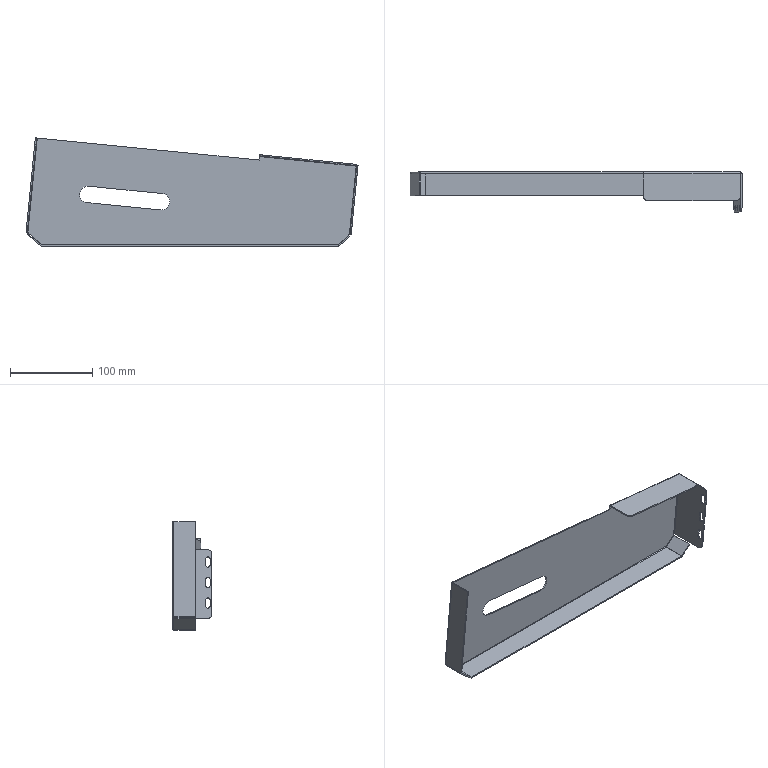Part | STEP file | 08-18 guard plate (Default) | 1 solid | 89 faces | box 402.823 x 48.5 x 131.437 mm | volume 95492 mm3 | plane 61 | cylinder 28 | commonest cylinder face diameters 5.5 x9 1.473 x6 4.473 x6 10 x4 20 x3